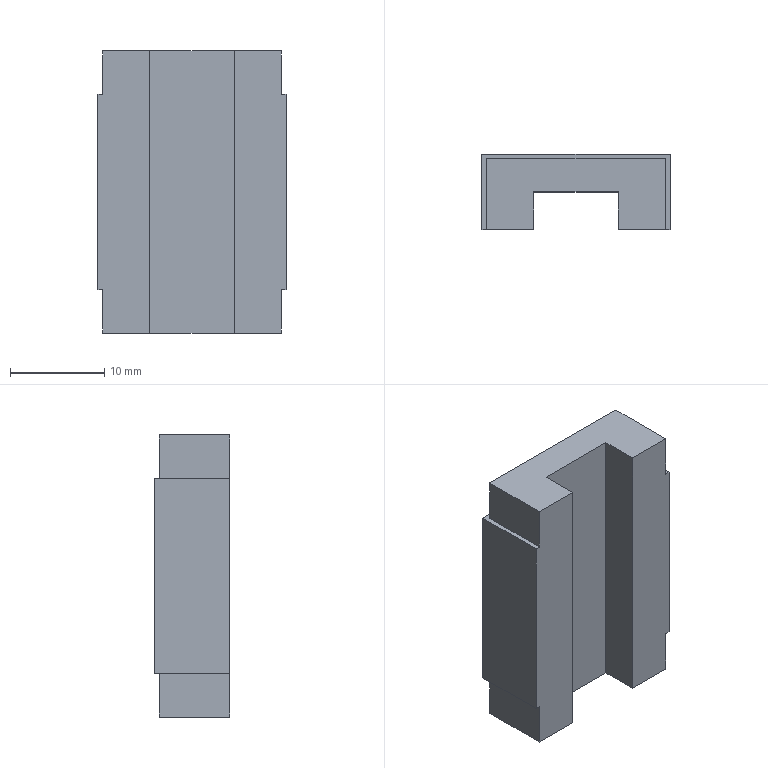Part | NX | features BREP 5 | 1 solid | 46 faces | box 20 x 8 x 30 mm | volume 3531 mm3 | plane 22 | cylinder 16 | cone 8 | commonest cylinder face diameters 2.5 x8 3 x8